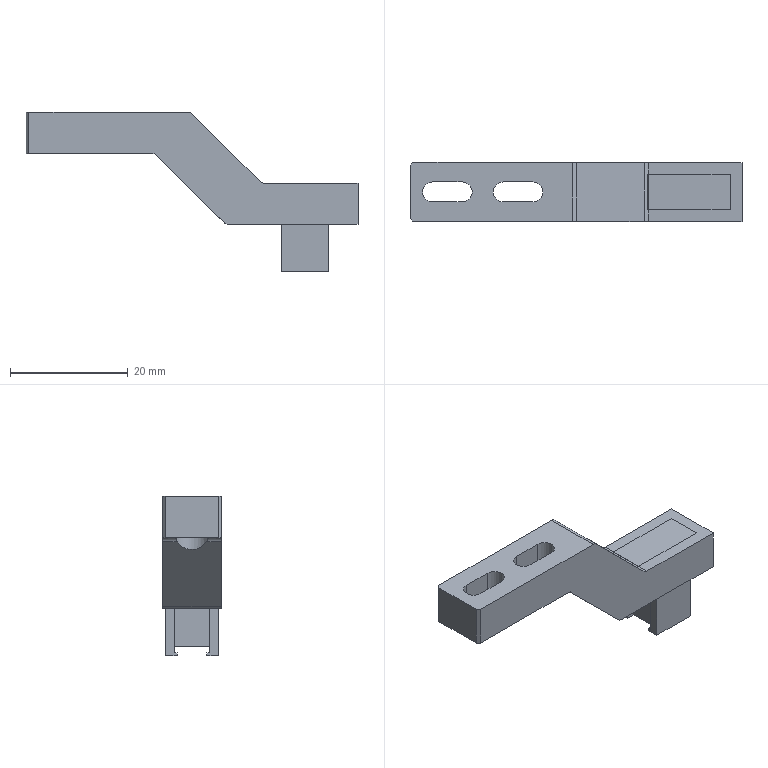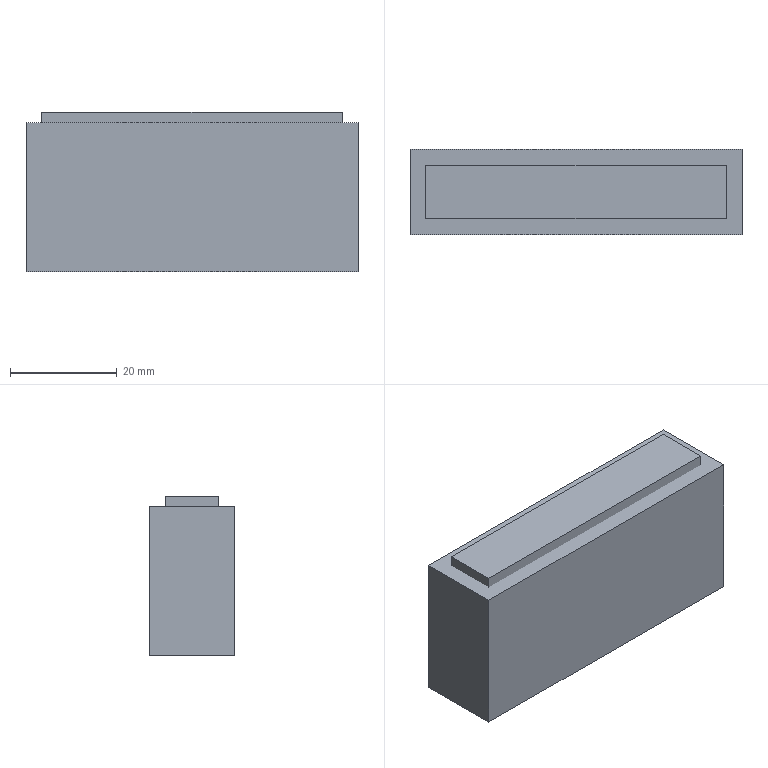CAM job | NX | 3-axis milling | part box 56.3 x 10 x 27 mm | stock box 62.3 x 16 x 30 mm
Tools:
number,name,description,diameter,corner_radius,flute_length,length,flutes
1,D63,Milling Tool-5 Parameters,63.0,0.0,50.0,75.0,2
10,D10,Milling Tool-5 Parameters,10.0,0.0,50.0,75.0,2
11,D10JING,Milling Tool-5 Parameters,10.0,0.0,50.0,75.0,2
6,D6,Milling Tool-5 Parameters,6.0,0.0,50.0,75.0,2
4,D4,Milling Tool-5 Parameters,4.0,0.0,50.0,75.0,2
5,D4R0.2,Milling Tool-5 Parameters,4.0,0.2,50.0,75.0,2
2,D2,Milling Tool-5 Parameters,2.0,0.0,50.0,75.0,2
7,D6A45,Milling Tool-5 Parameters,6.0,0.0,3.0,3.0,2
Operations:
program,operation,operation_type,tool,method,geometry_group,spindle_rpm,surface_speed,feed_per_tooth,feed_cut,feed_plunge,cut_length_mm,path_length_mm,cut_time_min,machine_time_min
1,FLOOR_WALL,VolumeBased25DMillingOperation,D63,METHOD,A,6500.0,1286.0,0.0962,1250.0,100.0,137.3,191.3,0.1098,0.1152
1,ADAPTIVE_MILLING,CavityMilling,D10,METHOD,A,9500.0,298.0,0.1579,3000.0,1000.0,2913.273,4262.008,0.9804,1.115
1,ZLEVEL_PROFILE_COPY_COPY_1,ZLevelMilling,D10JING,METHOD,A,9500.0,298.0,0.0632,1200.0,100.0,342.902,533.596,0.2858,0.3048
1,FLOOR_WALL_1,VolumeBased25DMillingOperation,D6,METHOD,A,9500.0,179.0,0.0658,1250.0,100.0,159.159,340.161,0.1273,0.1454
1,ZLEVEL_PROFILE,ZLevelMilling,D4,METHOD,A,9500.0,119.0,0.1053,2000.0,800.0,1483.665,1691.226,0.792,0.8127
1,ZLEVEL_PROFILE_COPY,ZLevelMilling,D4,METHOD,A,9500.0,119.0,0.0632,1200.0,800.0,275.079,370.579,0.2556,0.2652
1,ZLEVEL_PROFILE_COPY_COPY,ZLevelMilling,D4,METHOD,A,9500.0,119.0,0.0632,1200.0,800.0,62.975,173.475,0.0684,0.0795
1,ZLEVEL_PROFILE_COPY_1,ZLevelMilling,D4R0.2,METHOD,A,9500.0,119.0,0.1053,2000.0,800.0,2002.323,2071.336,1.003,1.01
1,ZLEVEL_PROFILE_COPY_2,ZLevelMilling,D2,METHOD,A,9500.0,59.0,0.0579,1100.0,800.0,1434.738,1577.869,1.326,1.34
1,ZLEVEL_PROFILE_1_COPY_1,ZLevelMilling,D6A45,METHOD,A,9500.0,179.0,0.0526,1000.0,100.0,108.344,307.246,0.1083,0.1282
1,ZLEVEL_PROFILE_1_COPY_1_COPY,ZLevelMilling,D6A45,METHOD,A,9500.0,179.0,0.0526,1000.0,100.0,82.368,256.789,0.0824,0.0998
2,FLOOR_WALL_COPY,VolumeBased25DMillingOperation,D63,METHOD,B,6500.0,1286.0,0.0962,1250.0,100.0,393.9,800.501,0.3151,0.3558
2,ADAPTIVE_MILLING_COPY,CavityMilling,D10,METHOD,B,9500.0,298.0,0.1579,3000.0,1000.0,1937.438,4509.579,0.6618,0.919
2,FLOOR_WALL_1_1,VolumeBased25DMillingOperation,D6,METHOD,B,9500.0,179.0,0.0658,1250.0,100.0,439.876,937.226,0.3519,0.4016
2,ZLEVEL_PROFILE_COPY_2_COPY,ZLevelMilling,D4,METHOD,B,9500.0,59.0,0.0579,1100.0,800.0,549.683,764.42,0.5224,0.5439
2,ZLEVEL_PROFILE_COPY_COPY_1_COPY,ZLevelMilling,D4,METHOD,B,9500.0,298.0,0.0632,1200.0,100.0,23.839,124.639,0.0199,0.0299
2,ZLEVEL_PROFILE_COPY_1_COPY,ZLevelMilling,D4R0.2,METHOD,B,9500.0,119.0,0.1053,2000.0,800.0,1931.858,2223.682,0.9717,1.001
2,ZLEVEL_PROFILE_1_COPY_1_COPY_1,ZLevelMilling,D6A45,METHOD,B,9500.0,179.0,0.0526,1000.0,100.0,62.242,197.541,0.0622,0.0758
2,ZLEVEL_PROFILE_1_COPY_1_COPY_1_COPY,ZLevelMilling,D6A45,METHOD,B,9500.0,179.0,0.0526,1000.0,100.0,108.193,426.313,0.1082,0.14
2,ZLEVEL_PROFILE_1_COPY_1_COPY_1_COPY_COPY,ZLevelMilling,D6A45,METHOD,B,9500.0,179.0,0.0526,1000.0,100.0,43.915,300.537,0.0439,0.0696